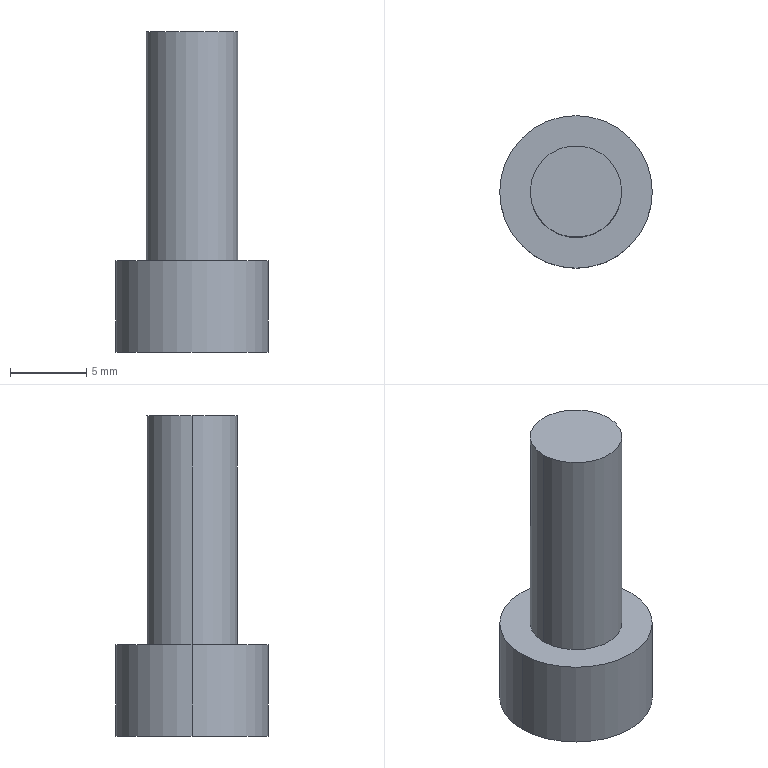Part | STEP file | LG M6_1.5F | 1 solid | 14 faces | box 10 x 10 x 21 mm | volume 829.881 mm3 | plane 10 | cylinder 4 | commonest cylinder face diameters 6 x2 10 x2
STEP:
#1=CARTESIAN_POINT('',(0.,0.,0.));
#2=DIRECTION('',(0.,0.,1.));
#3=DIRECTION('',(1.,0.,0.));
#4=AXIS2_PLACEMENT_3D('',#1,#2,#3);
#5=CARTESIAN_POINT('',(3.,0.,15.));
#6=VERTEX_POINT('',#5);
#7=CARTESIAN_POINT('',(-3.,0.,15.));
#8=VERTEX_POINT('',#7);
#9=CARTESIAN_POINT('',(0.,0.,15.));
#10=DIRECTION('',(0.,0.,1.));
#11=DIRECTION('',(1.,0.,0.));
#12=AXIS2_PLACEMENT_3D('',#9,#10,#11);
#13=CIRCLE('',#12,3.);
#14=CARTESIAN_POINT('',(0.,0.,15.));
#15=DIRECTION('',(0.,0.,-1.));
#16=DIRECTION('',(-1.,0.,0.));
#17=AXIS2_PLACEMENT_3D('',#14,#15,#16);
#18=CYLINDRICAL_SURFACE('',#17,3.);
#19=CARTESIAN_POINT('',(3.142,0.));
#20=DIRECTION('',(-1.,0.));
#21=VECTOR('',#20,1.);
#22=LINE('',#19,#21);
#23=(GEOMETRIC_REPRESENTATION_CONTEXT(2)PARAMETRIC_REPRESENTATION_CONTEXT()REPRESENTATION_CONTEXT('',''));
#24=DEFINITIONAL_REPRESENTATION('',(#22),#23);
#25=PCURVE('',#18,#24);
#26=CARTESIAN_POINT('',(0.,0.,15.));
#27=DIRECTION('',(0.,0.,1.));
#28=DIRECTION('',(1.,0.,0.));
#29=AXIS2_PLACEMENT_3D('',#26,#27,#28);
#30=PLANE('',#29);
#31=CARTESIAN_POINT('',(0.,0.));
#32=DIRECTION('',(1.,0.));
#33=AXIS2_PLACEMENT_2D('',#31,#32);
#34=CIRCLE('',#33,3.);
#35=(GEOMETRIC_REPRESENTATION_CONTEXT(2)PARAMETRIC_REPRESENTATION_CONTEXT()REPRESENTATION_CONTEXT('',''));
#36=DEFINITIONAL_REPRESENTATION('',(#34),#35);
#37=PCURVE('',#30,#36);
#38=SURFACE_CURVE('',#13,(#25,#37),.PCURVE_S1.);
#39=EDGE_CURVE('',#6,#8,#38,.T.);
#40=ORIENTED_EDGE('',*,*,#39,.F.);
#41=CARTESIAN_POINT('',(3.,0.,0.));
#42=VERTEX_POINT('',#41);
#43=CARTESIAN_POINT('',(3.,0.,15.));
#44=DIRECTION('',(0.,0.,-1.));
#45=VECTOR('',#44,1.);
#46=LINE('',#43,#45);
#47=CARTESIAN_POINT('',(3.142,0.));
#48=DIRECTION('',(0.,1.));
#49=VECTOR('',#48,1.);
#50=LINE('',#47,#49);
#51=(GEOMETRIC_REPRESENTATION_CONTEXT(2)PARAMETRIC_REPRESENTATION_CONTEXT()REPRESENTATION_CONTEXT('',''));
#52=DEFINITIONAL_REPRESENTATION('',(#50),#51);
#53=PCURVE('',#18,#52);
#54=CARTESIAN_POINT('',(0.,0.,15.));
#55=DIRECTION('',(0.,0.,-1.));
#56=DIRECTION('',(-1.,0.,0.));
#57=AXIS2_PLACEMENT_3D('',#54,#55,#56);
#58=CYLINDRICAL_SURFACE('',#57,3.);
#59=CARTESIAN_POINT('',(3.142,0.));
#60=DIRECTION('',(0.,1.));
#61=VECTOR('',#60,1.);
#62=LINE('',#59,#61);
#63=(GEOMETRIC_REPRESENTATION_CONTEXT(2)PARAMETRIC_REPRESENTATION_CONTEXT()REPRESENTATION_CONTEXT('',''));
#64=DEFINITIONAL_REPRESENTATION('',(#62),#63);
#65=PCURVE('',#58,#64);
#66=SURFACE_CURVE('',#46,(#53,#65),.PCURVE_S1.);
#67=EDGE_CURVE('',#6,#42,#66,.T.);
#68=ORIENTED_EDGE('',*,*,#67,.T.);
#69=CARTESIAN_POINT('',(-3.,0.,0.));
#70=VERTEX_POINT('',#69);
#71=CARTESIAN_POINT('',(0.,0.,0.));
#72=DIRECTION('',(0.,0.,1.));
#73=DIRECTION('',(1.,0.,0.));
#74=AXIS2_PLACEMENT_3D('',#71,#72,#73);
#75=CIRCLE('',#74,3.);
#76=CARTESIAN_POINT('',(3.142,15.));
#77=DIRECTION('',(-1.,0.));
#78=VECTOR('',#77,1.);
#79=LINE('',#76,#78);
#80=(GEOMETRIC_REPRESENTATION_CONTEXT(2)PARAMETRIC_REPRESENTATION_CONTEXT()REPRESENTATION_CONTEXT('',''));
#81=DEFINITIONAL_REPRESENTATION('',(#79),#80);
#82=PCURVE('',#18,#81);
#83=CARTESIAN_POINT('',(0.,0.,0.));
#84=DIRECTION('',(0.,0.,1.));
#85=DIRECTION('',(1.,0.,0.));
#86=AXIS2_PLACEMENT_3D('',#83,#84,#85);
#87=PLANE('',#86);
#88=CARTESIAN_POINT('',(0.,0.));
#89=DIRECTION('',(1.,0.));
#90=AXIS2_PLACEMENT_2D('',#88,#89);
#91=CIRCLE('',#90,3.);
#92=(GEOMETRIC_REPRESENTATION_CONTEXT(2)PARAMETRIC_REPRESENTATION_CONTEXT()REPRESENTATION_CONTEXT('',''));
#93=DEFINITIONAL_REPRESENTATION('',(#91),#92);
#94=PCURVE('',#87,#93);
#95=SURFACE_CURVE('',#75,(#82,#94),.PCURVE_S1.);
#96=EDGE_CURVE('',#42,#70,#95,.T.);
#97=ORIENTED_EDGE('',*,*,#96,.T.);
#98=CARTESIAN_POINT('',(-3.,0.,15.));
#99=DIRECTION('',(0.,0.,-1.));
#100=VECTOR('',#99,1.);
#101=LINE('',#98,#100);
#102=CARTESIAN_POINT('',(0.,0.));
#103=DIRECTION('',(0.,1.));
#104=VECTOR('',#103,1.);
#105=LINE('',#102,#104);
#106=(GEOMETRIC_REPRESENTATION_CONTEXT(2)PARAMETRIC_REPRESENTATION_CONTEXT()REPRESENTATION_CONTEXT('',''));
#107=DEFINITIONAL_REPRESENTATION('',(#105),#106);
#108=PCURVE('',#18,#107);
#109=CARTESIAN_POINT('',(6.283,0.));
#110=DIRECTION('',(0.,1.));
#111=VECTOR('',#110,1.);
#112=LINE('',#109,#111);
#113=(GEOMETRIC_REPRESENTATION_CONTEXT(2)PARAMETRIC_REPRESENTATION_CONTEXT()REPRESENTATION_CONTEXT('',''));
#114=DEFINITIONAL_REPRESENTATION('',(#112),#113);
#115=PCURVE('',#58,#114);
#116=SURFACE_CURVE('',#101,(#108,#115),.PCURVE_S1.);
#117=EDGE_CURVE('',#8,#70,#116,.T.);
#118=ORIENTED_EDGE('',*,*,#117,.F.);
#119=EDGE_LOOP('',(#40,#68,#97,#118));
#120=FACE_BOUND('',#119,.T.);
#121=ADVANCED_FACE('',(#120),#18,.T.);
#122=CARTESIAN_POINT('',(5.,0.,-6.));
#123=VERTEX_POINT('',#122);
#124=CARTESIAN_POINT('',(-5.,0.,-6.));
#125=VERTEX_POINT('',#124);
#126=CARTESIAN_POINT('',(0.,0.,-6.));
#127=DIRECTION('',(0.,0.,1.));
#128=DIRECTION('',(1.,0.,0.));
#129=AXIS2_PLACEMENT_3D('',#126,#127,#128);
#130=CIRCLE('',#129,5.);
#131=CARTESIAN_POINT('',(0.,0.,-6.));
#132=DIRECTION('',(0.,0.,1.));
#133=DIRECTION('',(1.,0.,0.));
#134=AXIS2_PLACEMENT_3D('',#131,#132,#133);
#135=CYLINDRICAL_SURFACE('',#134,5.);
#136=CARTESIAN_POINT('',(0.,0.));
#137=DIRECTION('',(1.,0.));
#138=VECTOR('',#137,1.);
#139=LINE('',#136,#138);
#140=(GEOMETRIC_REPRESENTATION_CONTEXT(2)PARAMETRIC_REPRESENTATION_CONTEXT()REPRESENTATION_CONTEXT('',''));
#141=DEFINITIONAL_REPRESENTATION('',(#139),#140);
#142=PCURVE('',#135,#141);
#143=CARTESIAN_POINT('',(0.,0.,-6.));
#144=DIRECTION('',(0.,0.,1.));
#145=DIRECTION('',(1.,0.,0.));
#146=AXIS2_PLACEMENT_3D('',#143,#144,#145);
#147=PLANE('',#146);
#148=CARTESIAN_POINT('',(0.,0.));
#149=DIRECTION('',(1.,0.));
#150=AXIS2_PLACEMENT_2D('',#148,#149);
#151=CIRCLE('',#150,5.);
#152=(GEOMETRIC_REPRESENTATION_CONTEXT(2)PARAMETRIC_REPRESENTATION_CONTEXT()REPRESENTATION_CONTEXT('',''));
#153=DEFINITIONAL_REPRESENTATION('',(#151),#152);
#154=PCURVE('',#147,#153);
#155=SURFACE_CURVE('',#130,(#142,#154),.PCURVE_S1.);
#156=EDGE_CURVE('',#123,#125,#155,.T.);
#157=ORIENTED_EDGE('',*,*,#156,.T.);
#158=CARTESIAN_POINT('',(-5.,0.,0.));
#159=VERTEX_POINT('',#158);
#160=CARTESIAN_POINT('',(-5.,0.,-6.));
#161=DIRECTION('',(0.,0.,1.));
#162=VECTOR('',#161,1.);
#163=LINE('',#160,#162);
#164=CARTESIAN_POINT('',(3.142,0.));
#165=DIRECTION('',(0.,1.));
#166=VECTOR('',#165,1.);
#167=LINE('',#164,#166);
#168=(GEOMETRIC_REPRESENTATION_CONTEXT(2)PARAMETRIC_REPRESENTATION_CONTEXT()REPRESENTATION_CONTEXT('',''));
#169=DEFINITIONAL_REPRESENTATION('',(#167),#168);
#170=PCURVE('',#135,#169);
#171=CARTESIAN_POINT('',(0.,0.,-6.));
#172=DIRECTION('',(0.,0.,1.));
#173=DIRECTION('',(1.,0.,0.));
#174=AXIS2_PLACEMENT_3D('',#171,#172,#173);
#175=CYLINDRICAL_SURFACE('',#174,5.);
#176=CARTESIAN_POINT('',(3.142,0.));
#177=DIRECTION('',(0.,1.));
#178=VECTOR('',#177,1.);
#179=LINE('',#176,#178);
#180=(GEOMETRIC_REPRESENTATION_CONTEXT(2)PARAMETRIC_REPRESENTATION_CONTEXT()REPRESENTATION_CONTEXT('',''));
#181=DEFINITIONAL_REPRESENTATION('',(#179),#180);
#182=PCURVE('',#175,#181);
#183=SURFACE_CURVE('',#163,(#170,#182),.PCURVE_S1.);
#184=EDGE_CURVE('',#125,#159,#183,.T.);
#185=ORIENTED_EDGE('',*,*,#184,.T.);
#186=CARTESIAN_POINT('',(5.,0.,0.));
#187=VERTEX_POINT('',#186);
#188=CARTESIAN_POINT('',(0.,0.,0.));
#189=DIRECTION('',(0.,0.,1.));
#190=DIRECTION('',(1.,0.,0.));
#191=AXIS2_PLACEMENT_3D('',#188,#189,#190);
#192=CIRCLE('',#191,5.);
#193=CARTESIAN_POINT('',(0.,6.));
#194=DIRECTION('',(1.,0.));
#195=VECTOR('',#194,1.);
#196=LINE('',#193,#195);
#197=(GEOMETRIC_REPRESENTATION_CONTEXT(2)PARAMETRIC_REPRESENTATION_CONTEXT()REPRESENTATION_CONTEXT('',''));
#198=DEFINITIONAL_REPRESENTATION('',(#196),#197);
#199=PCURVE('',#135,#198);
#200=CARTESIAN_POINT('',(0.,0.));
#201=DIRECTION('',(1.,0.));
#202=AXIS2_PLACEMENT_2D('',#200,#201);
#203=CIRCLE('',#202,5.);
#204=(GEOMETRIC_REPRESENTATION_CONTEXT(2)PARAMETRIC_REPRESENTATION_CONTEXT()REPRESENTATION_CONTEXT('',''));
#205=DEFINITIONAL_REPRESENTATION('',(#203),#204);
#206=PCURVE('',#87,#205);
#207=SURFACE_CURVE('',#192,(#199,#206),.PCURVE_S1.);
#208=EDGE_CURVE('',#187,#159,#207,.T.);
#209=ORIENTED_EDGE('',*,*,#208,.F.);
#210=CARTESIAN_POINT('',(5.,0.,-6.));
#211=DIRECTION('',(0.,0.,1.));
#212=VECTOR('',#211,1.);
#213=LINE('',#210,#212);
#214=CARTESIAN_POINT('',(0.,0.));
#215=DIRECTION('',(0.,1.));
#216=VECTOR('',#215,1.);
#217=LINE('',#214,#216);
#218=(GEOMETRIC_REPRESENTATION_CONTEXT(2)PARAMETRIC_REPRESENTATION_CONTEXT()REPRESENTATION_CONTEXT('',''));
#219=DEFINITIONAL_REPRESENTATION('',(#217),#218);
#220=PCURVE('',#135,#219);
#221=CARTESIAN_POINT('',(6.283,0.));
#222=DIRECTION('',(0.,1.));
#223=VECTOR('',#222,1.);
#224=LINE('',#221,#223);
#225=(GEOMETRIC_REPRESENTATION_CONTEXT(2)PARAMETRIC_REPRESENTATION_CONTEXT()REPRESENTATION_CONTEXT('',''));
#226=DEFINITIONAL_REPRESENTATION('',(#224),#225);
#227=PCURVE('',#175,#226);
#228=SURFACE_CURVE('',#213,(#220,#227),.PCURVE_S1.);
#229=EDGE_CURVE('',#123,#187,#228,.T.);
#230=ORIENTED_EDGE('',*,*,#229,.F.);
#231=EDGE_LOOP('',(#157,#185,#209,#230));
#232=FACE_BOUND('',#231,.T.);
#233=ADVANCED_FACE('',(#232),#135,.T.);
#234=ORIENTED_EDGE('',*,*,#208,.T.);
#235=CARTESIAN_POINT('',(0.,0.,0.));
#236=DIRECTION('',(0.,0.,1.));
#237=DIRECTION('',(1.,0.,0.));
#238=AXIS2_PLACEMENT_3D('',#235,#236,#237);
#239=CIRCLE('',#238,5.);
#240=CARTESIAN_POINT('',(0.,0.));
#241=DIRECTION('',(1.,0.));
#242=AXIS2_PLACEMENT_2D('',#240,#241);
#243=CIRCLE('',#242,5.);
#244=(GEOMETRIC_REPRESENTATION_CONTEXT(2)PARAMETRIC_REPRESENTATION_CONTEXT()REPRESENTATION_CONTEXT('',''));
#245=DEFINITIONAL_REPRESENTATION('',(#243),#244);
#246=PCURVE('',#87,#245);
#247=CARTESIAN_POINT('',(0.,6.));
#248=DIRECTION('',(1.,0.));
#249=VECTOR('',#248,1.);
#250=LINE('',#247,#249);
#251=(GEOMETRIC_REPRESENTATION_CONTEXT(2)PARAMETRIC_REPRESENTATION_CONTEXT()REPRESENTATION_CONTEXT('',''));
#252=DEFINITIONAL_REPRESENTATION('',(#250),#251);
#253=PCURVE('',#175,#252);
#254=SURFACE_CURVE('',#239,(#246,#253),.PCURVE_S1.);
#255=EDGE_CURVE('',#159,#187,#254,.T.);
#256=ORIENTED_EDGE('',*,*,#255,.T.);
#257=EDGE_LOOP('',(#234,#256));
#258=FACE_BOUND('',#257,.T.);
#259=CARTESIAN_POINT('',(0.,0.,0.));
#260=DIRECTION('',(0.,0.,1.));
#261=DIRECTION('',(1.,0.,0.));
#262=AXIS2_PLACEMENT_3D('',#259,#260,#261);
#263=CIRCLE('',#262,3.);
#264=CARTESIAN_POINT('',(0.,0.));
#265=DIRECTION('',(1.,0.));
#266=AXIS2_PLACEMENT_2D('',#264,#265);
#267=CIRCLE('',#266,3.);
#268=(GEOMETRIC_REPRESENTATION_CONTEXT(2)PARAMETRIC_REPRESENTATION_CONTEXT()REPRESENTATION_CONTEXT('',''));
#269=DEFINITIONAL_REPRESENTATION('',(#267),#268);
#270=PCURVE('',#87,#269);
#271=CARTESIAN_POINT('',(9.425,15.));
#272=DIRECTION('',(-1.,0.));
#273=VECTOR('',#272,1.);
#274=LINE('',#271,#273);
#275=(GEOMETRIC_REPRESENTATION_CONTEXT(2)PARAMETRIC_REPRESENTATION_CONTEXT()REPRESENTATION_CONTEXT('',''));
#276=DEFINITIONAL_REPRESENTATION('',(#274),#275);
#277=PCURVE('',#58,#276);
#278=SURFACE_CURVE('',#263,(#270,#277),.PCURVE_S1.);
#279=EDGE_CURVE('',#70,#42,#278,.T.);
#280=ORIENTED_EDGE('',*,*,#279,.F.);
#281=ORIENTED_EDGE('',*,*,#96,.F.);
#282=EDGE_LOOP('',(#280,#281));
#283=FACE_BOUND('',#282,.T.);
#284=ADVANCED_FACE('',(#258,#283),#87,.T.);
#285=ORIENTED_EDGE('',*,*,#184,.F.);
#286=CARTESIAN_POINT('',(0.,0.,-6.));
#287=DIRECTION('',(0.,0.,1.));
#288=DIRECTION('',(1.,0.,0.));
#289=AXIS2_PLACEMENT_3D('',#286,#287,#288);
#290=CIRCLE('',#289,5.);
#291=CARTESIAN_POINT('',(0.,0.));
#292=DIRECTION('',(1.,0.));
#293=VECTOR('',#292,1.);
#294=LINE('',#291,#293);
#295=(GEOMETRIC_REPRESENTATION_CONTEXT(2)PARAMETRIC_REPRESENTATION_CONTEXT()REPRESENTATION_CONTEXT('',''));
#296=DEFINITIONAL_REPRESENTATION('',(#294),#295);
#297=PCURVE('',#175,#296);
#298=CARTESIAN_POINT('',(0.,0.));
#299=DIRECTION('',(1.,0.));
#300=AXIS2_PLACEMENT_2D('',#298,#299);
#301=CIRCLE('',#300,5.);
#302=(GEOMETRIC_REPRESENTATION_CONTEXT(2)PARAMETRIC_REPRESENTATION_CONTEXT()REPRESENTATION_CONTEXT('',''));
#303=DEFINITIONAL_REPRESENTATION('',(#301),#302);
#304=PCURVE('',#147,#303);
#305=SURFACE_CURVE('',#290,(#297,#304),.PCURVE_S1.);
#306=EDGE_CURVE('',#125,#123,#305,.T.);
#307=ORIENTED_EDGE('',*,*,#306,.T.);
#308=ORIENTED_EDGE('',*,*,#229,.T.);
#309=ORIENTED_EDGE('',*,*,#255,.F.);
#310=EDGE_LOOP('',(#285,#307,#308,#309));
#311=FACE_BOUND('',#310,.T.);
#312=ADVANCED_FACE('',(#311),#175,.T.);
#313=CARTESIAN_POINT('',(-2.898,0.,-6.));
#314=VERTEX_POINT('',#313);
#315=CARTESIAN_POINT('',(-1.449,2.51,-6.));
#316=VERTEX_POINT('',#315);
#317=CARTESIAN_POINT('',(-2.898,0.,-6.));
#318=DIRECTION('',(0.5,0.866,0.));
#319=VECTOR('',#318,1.);
#320=LINE('',#317,#319);
#321=CARTESIAN_POINT('',(-2.898,0.));
#322=DIRECTION('',(0.5,0.866));
#323=VECTOR('',#322,1.);
#324=LINE('',#321,#323);
#325=(GEOMETRIC_REPRESENTATION_CONTEXT(2)PARAMETRIC_REPRESENTATION_CONTEXT()REPRESENTATION_CONTEXT('',''));
#326=DEFINITIONAL_REPRESENTATION('',(#324),#325);
#327=PCURVE('',#147,#326);
#328=CARTESIAN_POINT('',(-2.898,0.,-3.));
#329=DIRECTION('',(-0.866,0.5,0.));
#330=DIRECTION('',(-0.5,-0.866,0.));
#331=AXIS2_PLACEMENT_3D('',#328,#329,#330);
#332=PLANE('',#331);
#333=CARTESIAN_POINT('',(0.,-3.));
#334=DIRECTION('',(-1.,0.));
#335=VECTOR('',#334,1.);
#336=LINE('',#333,#335);
#337=(GEOMETRIC_REPRESENTATION_CONTEXT(2)PARAMETRIC_REPRESENTATION_CONTEXT()REPRESENTATION_CONTEXT('',''));
#338=DEFINITIONAL_REPRESENTATION('',(#336),#337);
#339=PCURVE('',#332,#338);
#340=SURFACE_CURVE('',#320,(#327,#339),.PCURVE_S1.);
#341=EDGE_CURVE('',#314,#316,#340,.T.);
#342=ORIENTED_EDGE('',*,*,#341,.F.);
#343=CARTESIAN_POINT('',(-1.449,-2.51,-6.));
#344=VERTEX_POINT('',#343);
#345=CARTESIAN_POINT('',(-1.449,-2.51,-6.));
#346=DIRECTION('',(-0.5,0.866,0.));
#347=VECTOR('',#346,1.);
#348=LINE('',#345,#347);
#349=CARTESIAN_POINT('',(-1.449,-2.51));
#350=DIRECTION('',(-0.5,0.866));
#351=VECTOR('',#350,1.);
#352=LINE('',#349,#351);
#353=(GEOMETRIC_REPRESENTATION_CONTEXT(2)PARAMETRIC_REPRESENTATION_CONTEXT()REPRESENTATION_CONTEXT('',''));
#354=DEFINITIONAL_REPRESENTATION('',(#352),#353);
#355=PCURVE('',#147,#354);
#356=CARTESIAN_POINT('',(-1.449,-2.51,-3.));
#357=DIRECTION('',(-0.866,-0.5,0.));
#358=DIRECTION('',(0.5,-0.866,0.));
#359=AXIS2_PLACEMENT_3D('',#356,#357,#358);
#360=PLANE('',#359);
#361=CARTESIAN_POINT('',(0.,-3.));
#362=DIRECTION('',(-1.,0.));
#363=VECTOR('',#362,1.);
#364=LINE('',#361,#363);
#365=(GEOMETRIC_REPRESENTATION_CONTEXT(2)PARAMETRIC_REPRESENTATION_CONTEXT()REPRESENTATION_CONTEXT('',''));
#366=DEFINITIONAL_REPRESENTATION('',(#364),#365);
#367=PCURVE('',#360,#366);
#368=SURFACE_CURVE('',#348,(#355,#367),.PCURVE_S1.);
#369=EDGE_CURVE('',#344,#314,#368,.T.);
#370=ORIENTED_EDGE('',*,*,#369,.F.);
#371=CARTESIAN_POINT('',(1.449,-2.51,-6.));
#372=VERTEX_POINT('',#371);
#373=CARTESIAN_POINT('',(1.449,-2.51,-6.));
#374=DIRECTION('',(-1.,0.,0.));
#375=VECTOR('',#374,1.);
#376=LINE('',#373,#375);
#377=CARTESIAN_POINT('',(1.449,-2.51));
#378=DIRECTION('',(-1.,0.));
#379=VECTOR('',#378,1.);
#380=LINE('',#377,#379);
#381=(GEOMETRIC_REPRESENTATION_CONTEXT(2)PARAMETRIC_REPRESENTATION_CONTEXT()REPRESENTATION_CONTEXT('',''));
#382=DEFINITIONAL_REPRESENTATION('',(#380),#381);
#383=PCURVE('',#147,#382);
#384=CARTESIAN_POINT('',(1.449,-2.51,-3.));
#385=DIRECTION('',(0.,-1.,0.));
#386=DIRECTION('',(0.,0.,-1.));
#387=AXIS2_PLACEMENT_3D('',#384,#385,#386);
#388=PLANE('',#387);
#389=CARTESIAN_POINT('',(3.,0.));
#390=DIRECTION('',(0.,-1.));
#391=VECTOR('',#390,1.);
#392=LINE('',#389,#391);
#393=(GEOMETRIC_REPRESENTATION_CONTEXT(2)PARAMETRIC_REPRESENTATION_CONTEXT()REPRESENTATION_CONTEXT('',''));
#394=DEFINITIONAL_REPRESENTATION('',(#392),#393);
#395=PCURVE('',#388,#394);
#396=SURFACE_CURVE('',#376,(#383,#395),.PCURVE_S1.);
#397=EDGE_CURVE('',#372,#344,#396,.T.);
#398=ORIENTED_EDGE('',*,*,#397,.F.);
#399=CARTESIAN_POINT('',(2.898,0.,-6.));
#400=VERTEX_POINT('',#399);
#401=CARTESIAN_POINT('',(2.898,0.,-6.));
#402=DIRECTION('',(-0.5,-0.866,0.));
#403=VECTOR('',#402,1.);
#404=LINE('',#401,#403);
#405=CARTESIAN_POINT('',(2.898,0.));
#406=DIRECTION('',(-0.5,-0.866));
#407=VECTOR('',#406,1.);
#408=LINE('',#405,#407);
#409=(GEOMETRIC_REPRESENTATION_CONTEXT(2)PARAMETRIC_REPRESENTATION_CONTEXT()REPRESENTATION_CONTEXT('',''));
#410=DEFINITIONAL_REPRESENTATION('',(#408),#409);
#411=PCURVE('',#147,#410);
#412=CARTESIAN_POINT('',(2.898,0.,-3.));
#413=DIRECTION('',(0.866,-0.5,0.));
#414=DIRECTION('',(0.5,0.866,0.));
#415=AXIS2_PLACEMENT_3D('',#412,#413,#414);
#416=PLANE('',#415);
#417=CARTESIAN_POINT('',(0.,-3.));
#418=DIRECTION('',(-1.,0.));
#419=VECTOR('',#418,1.);
#420=LINE('',#417,#419);
#421=(GEOMETRIC_REPRESENTATION_CONTEXT(2)PARAMETRIC_REPRESENTATION_CONTEXT()REPRESENTATION_CONTEXT('',''));
#422=DEFINITIONAL_REPRESENTATION('',(#420),#421);
#423=PCURVE('',#416,#422);
#424=SURFACE_CURVE('',#404,(#411,#423),.PCURVE_S1.);
#425=EDGE_CURVE('',#400,#372,#424,.T.);
#426=ORIENTED_EDGE('',*,*,#425,.F.);
#427=CARTESIAN_POINT('',(1.449,2.51,-6.));
#428=VERTEX_POINT('',#427);
#429=CARTESIAN_POINT('',(1.449,2.51,-6.));
#430=DIRECTION('',(0.5,-0.866,0.));
#431=VECTOR('',#430,1.);
#432=LINE('',#429,#431);
#433=CARTESIAN_POINT('',(1.449,2.51));
#434=DIRECTION('',(0.5,-0.866));
#435=VECTOR('',#434,1.);
#436=LINE('',#433,#435);
#437=(GEOMETRIC_REPRESENTATION_CONTEXT(2)PARAMETRIC_REPRESENTATION_CONTEXT()REPRESENTATION_CONTEXT('',''));
#438=DEFINITIONAL_REPRESENTATION('',(#436),#437);
#439=PCURVE('',#147,#438);
#440=CARTESIAN_POINT('',(1.449,2.51,-3.));
#441=DIRECTION('',(0.866,0.5,0.));
#442=DIRECTION('',(-0.5,0.866,0.));
#443=AXIS2_PLACEMENT_3D('',#440,#441,#442);
#444=PLANE('',#443);
#445=CARTESIAN_POINT('',(0.,-3.));
#446=DIRECTION('',(-1.,0.));
#447=VECTOR('',#446,1.);
#448=LINE('',#445,#447);
#449=(GEOMETRIC_REPRESENTATION_CONTEXT(2)PARAMETRIC_REPRESENTATION_CONTEXT()REPRESENTATION_CONTEXT('',''));
#450=DEFINITIONAL_REPRESENTATION('',(#448),#449);
#451=PCURVE('',#444,#450);
#452=SURFACE_CURVE('',#432,(#439,#451),.PCURVE_S1.);
#453=EDGE_CURVE('',#428,#400,#452,.T.);
#454=ORIENTED_EDGE('',*,*,#453,.F.);
#455=CARTESIAN_POINT('',(-1.449,2.51,-6.));
#456=DIRECTION('',(1.,0.,0.));
#457=VECTOR('',#456,1.);
#458=LINE('',#455,#457);
#459=CARTESIAN_POINT('',(-1.449,2.51));
#460=DIRECTION('',(1.,0.));
#461=VECTOR('',#460,1.);
#462=LINE('',#459,#461);
#463=(GEOMETRIC_REPRESENTATION_CONTEXT(2)PARAMETRIC_REPRESENTATION_CONTEXT()REPRESENTATION_CONTEXT('',''));
#464=DEFINITIONAL_REPRESENTATION('',(#462),#463);
#465=PCURVE('',#147,#464);
#466=CARTESIAN_POINT('',(-1.449,2.51,-3.));
#467=DIRECTION('',(0.,1.,0.));
#468=DIRECTION('',(0.,0.,1.));
#469=AXIS2_PLACEMENT_3D('',#466,#467,#468);
#470=PLANE('',#469);
#471=CARTESIAN_POINT('',(-3.,0.));
#472=DIRECTION('',(0.,1.));
#473=VECTOR('',#472,1.);
#474=LINE('',#471,#473);
#475=(GEOMETRIC_REPRESENTATION_CONTEXT(2)PARAMETRIC_REPRESENTATION_CONTEXT()REPRESENTATION_CONTEXT('',''));
#476=DEFINITIONAL_REPRESENTATION('',(#474),#475);
#477=PCURVE('',#470,#476);
#478=SURFACE_CURVE('',#458,(#465,#477),.PCURVE_S1.);
#479=EDGE_CURVE('',#316,#428,#478,.T.);
#480=ORIENTED_EDGE('',*,*,#479,.F.);
#481=EDGE_LOOP('',(#342,#370,#398,#426,#454,#480));
#482=FACE_BOUND('',#481,.T.);
#483=ORIENTED_EDGE('',*,*,#156,.F.);
#484=ORIENTED_EDGE('',*,*,#306,.F.);
#485=EDGE_LOOP('',(#483,#484));
#486=FACE_BOUND('',#485,.T.);
#487=ADVANCED_FACE('',(#482,#486),#147,.F.);
#488=ORIENTED_EDGE('',*,*,#67,.F.);
#489=CARTESIAN_POINT('',(0.,0.,15.));
#490=DIRECTION('',(0.,0.,1.));
#491=DIRECTION('',(1.,0.,0.));
#492=AXIS2_PLACEMENT_3D('',#489,#490,#491);
#493=CIRCLE('',#492,3.);
#494=CARTESIAN_POINT('',(9.425,0.));
#495=DIRECTION('',(-1.,0.));
#496=VECTOR('',#495,1.);
#497=LINE('',#494,#496);
#498=(GEOMETRIC_REPRESENTATION_CONTEXT(2)PARAMETRIC_REPRESENTATION_CONTEXT()REPRESENTATION_CONTEXT('',''));
#499=DEFINITIONAL_REPRESENTATION('',(#497),#498);
#500=PCURVE('',#58,#499);
#501=CARTESIAN_POINT('',(0.,0.));
#502=DIRECTION('',(1.,0.));
#503=AXIS2_PLACEMENT_2D('',#501,#502);
#504=CIRCLE('',#503,3.);
#505=(GEOMETRIC_REPRESENTATION_CONTEXT(2)PARAMETRIC_REPRESENTATION_CONTEXT()REPRESENTATION_CONTEXT('',''));
#506=DEFINITIONAL_REPRESENTATION('',(#504),#505);
#507=PCURVE('',#30,#506);
#508=SURFACE_CURVE('',#493,(#500,#507),.PCURVE_S1.);
#509=EDGE_CURVE('',#8,#6,#508,.T.);
#510=ORIENTED_EDGE('',*,*,#509,.F.);
#511=ORIENTED_EDGE('',*,*,#117,.T.);
#512=ORIENTED_EDGE('',*,*,#279,.T.);
#513=EDGE_LOOP('',(#488,#510,#511,#512));
#514=FACE_BOUND('',#513,.T.);
#515=ADVANCED_FACE('',(#514),#58,.T.);
#516=ORIENTED_EDGE('',*,*,#509,.T.);
#517=ORIENTED_EDGE('',*,*,#39,.T.);
#518=EDGE_LOOP('',(#516,#517));
#519=FACE_BOUND('',#518,.T.);
#520=ADVANCED_FACE('',(#519),#30,.T.);
#521=ORIENTED_EDGE('',*,*,#369,.T.);
#522=CARTESIAN_POINT('',(-2.898,0.,-3.));
#523=VERTEX_POINT('',#522);
#524=CARTESIAN_POINT('',(-2.898,0.,-3.));
#525=DIRECTION('',(0.,0.,-1.));
#526=VECTOR('',#525,1.);
#527=LINE('',#524,#526);
#528=CARTESIAN_POINT('',(-2.898,0.));
#529=DIRECTION('',(0.,-1.));
#530=VECTOR('',#529,1.);
#531=LINE('',#528,#530);
#532=(GEOMETRIC_REPRESENTATION_CONTEXT(2)PARAMETRIC_REPRESENTATION_CONTEXT()REPRESENTATION_CONTEXT('',''));
#533=DEFINITIONAL_REPRESENTATION('',(#531),#532);
#534=PCURVE('',#360,#533);
#535=CARTESIAN_POINT('',(0.,0.));
#536=DIRECTION('',(0.,-1.));
#537=VECTOR('',#536,1.);
#538=LINE('',#535,#537);
#539=(GEOMETRIC_REPRESENTATION_CONTEXT(2)PARAMETRIC_REPRESENTATION_CONTEXT()REPRESENTATION_CONTEXT('',''));
#540=DEFINITIONAL_REPRESENTATION('',(#538),#539);
#541=PCURVE('',#332,#540);
#542=SURFACE_CURVE('',#527,(#534,#541),.PCURVE_S1.);
#543=EDGE_CURVE('',#523,#314,#542,.T.);
#544=ORIENTED_EDGE('',*,*,#543,.F.);
#545=CARTESIAN_POINT('',(-1.449,-2.51,-3.));
#546=VERTEX_POINT('',#545);
#547=CARTESIAN_POINT('',(-1.449,-2.51,-3.));
#548=DIRECTION('',(-0.5,0.866,0.));
#549=VECTOR('',#548,1.);
#550=LINE('',#547,#549);
#551=CARTESIAN_POINT('',(0.,0.));
#552=DIRECTION('',(-1.,0.));
#553=VECTOR('',#552,1.);
#554=LINE('',#551,#553);
#555=(GEOMETRIC_REPRESENTATION_CONTEXT(2)PARAMETRIC_REPRESENTATION_CONTEXT()REPRESENTATION_CONTEXT('',''));
#556=DEFINITIONAL_REPRESENTATION('',(#554),#555);
#557=PCURVE('',#360,#556);
#558=CARTESIAN_POINT('',(0.,0.,-3.));
#559=DIRECTION('',(0.,0.,-1.));
#560=DIRECTION('',(-1.,0.,0.));
#561=AXIS2_PLACEMENT_3D('',#558,#559,#560);
#562=PLANE('',#561);
#563=CARTESIAN_POINT('',(1.449,-2.51));
#564=DIRECTION('',(0.5,0.866));
#565=VECTOR('',#564,1.);
#566=LINE('',#563,#565);
#567=(GEOMETRIC_REPRESENTATION_CONTEXT(2)PARAMETRIC_REPRESENTATION_CONTEXT()REPRESENTATION_CONTEXT('',''));
#568=DEFINITIONAL_REPRESENTATION('',(#566),#567);
#569=PCURVE('',#562,#568);
#570=SURFACE_CURVE('',#550,(#557,#569),.PCURVE_S1.);
#571=EDGE_CURVE('',#546,#523,#570,.T.);
#572=ORIENTED_EDGE('',*,*,#571,.F.);
#573=CARTESIAN_POINT('',(-1.449,-2.51,-3.));
#574=DIRECTION('',(0.,0.,-1.));
#575=VECTOR('',#574,1.);
#576=LINE('',#573,#575);
#577=CARTESIAN_POINT('',(0.,0.));
#578=DIRECTION('',(0.,-1.));
#579=VECTOR('',#578,1.);
#580=LINE('',#577,#579);
#581=(GEOMETRIC_REPRESENTATION_CONTEXT(2)PARAMETRIC_REPRESENTATION_CONTEXT()REPRESENTATION_CONTEXT('',''));
#582=DEFINITIONAL_REPRESENTATION('',(#580),#581);
#583=PCURVE('',#360,#582);
#584=CARTESIAN_POINT('',(0.,-2.898));
#585=DIRECTION('',(1.,0.));
#586=VECTOR('',#585,1.);
#587=LINE('',#584,#586);
#588=(GEOMETRIC_REPRESENTATION_CONTEXT(2)PARAMETRIC_REPRESENTATION_CONTEXT()REPRESENTATION_CONTEXT('',''));
#589=DEFINITIONAL_REPRESENTATION('',(#587),#588);
#590=PCURVE('',#388,#589);
#591=SURFACE_CURVE('',#576,(#583,#590),.PCURVE_S1.);
#592=EDGE_CURVE('',#546,#344,#591,.T.);
#593=ORIENTED_EDGE('',*,*,#592,.T.);
#594=EDGE_LOOP('',(#521,#544,#572,#593));
#595=FACE_BOUND('',#594,.T.);
#596=ADVANCED_FACE('',(#595),#360,.F.);
#597=ORIENTED_EDGE('',*,*,#397,.T.);
#598=ORIENTED_EDGE('',*,*,#592,.F.);
#599=CARTESIAN_POINT('',(1.449,-2.51,-3.));
#600=VERTEX_POINT('',#599);
#601=CARTESIAN_POINT('',(1.449,-2.51,-3.));
#602=DIRECTION('',(-1.,0.,0.));
#603=VECTOR('',#602,1.);
#604=LINE('',#601,#603);
#605=CARTESIAN_POINT('',(0.,0.));
#606=DIRECTION('',(0.,-1.));
#607=VECTOR('',#606,1.);
#608=LINE('',#605,#607);
#609=(GEOMETRIC_REPRESENTATION_CONTEXT(2)PARAMETRIC_REPRESENTATION_CONTEXT()REPRESENTATION_CONTEXT('',''));
#610=DEFINITIONAL_REPRESENTATION('',(#608),#609);
#611=PCURVE('',#388,#610);
#612=CARTESIAN_POINT('',(-1.449,-2.51));
#613=DIRECTION('',(1.,0.));
#614=VECTOR('',#613,1.);
#615=LINE('',#612,#614);
#616=(GEOMETRIC_REPRESENTATION_CONTEXT(2)PARAMETRIC_REPRESENTATION_CONTEXT()REPRESENTATION_CONTEXT('',''));
#617=DEFINITIONAL_REPRESENTATION('',(#615),#616);
#618=PCURVE('',#562,#617);
#619=SURFACE_CURVE('',#604,(#611,#618),.PCURVE_S1.);
#620=EDGE_CURVE('',#600,#546,#619,.T.);
#621=ORIENTED_EDGE('',*,*,#620,.F.);
#622=CARTESIAN_POINT('',(1.449,-2.51,-3.));
#623=DIRECTION('',(0.,0.,-1.));
#624=VECTOR('',#623,1.);
#625=LINE('',#622,#624);
#626=CARTESIAN_POINT('',(0.,0.));
#627=DIRECTION('',(1.,0.));
#628=VECTOR('',#627,1.);
#629=LINE('',#626,#628);
#630=(GEOMETRIC_REPRESENTATION_CONTEXT(2)PARAMETRIC_REPRESENTATION_CONTEXT()REPRESENTATION_CONTEXT('',''));
#631=DEFINITIONAL_REPRESENTATION('',(#629),#630);
#632=PCURVE('',#388,#631);
#633=CARTESIAN_POINT('',(-2.898,0.));
#634=DIRECTION('',(0.,-1.));
#635=VECTOR('',#634,1.);
#636=LINE('',#633,#635);
#637=(GEOMETRIC_REPRESENTATION_CONTEXT(2)PARAMETRIC_REPRESENTATION_CONTEXT()REPRESENTATION_CONTEXT('',''));
#638=DEFINITIONAL_REPRESENTATION('',(#636),#637);
#639=PCURVE('',#416,#638);
#640=SURFACE_CURVE('',#625,(#632,#639),.PCURVE_S1.);
#641=EDGE_CURVE('',#600,#372,#640,.T.);
#642=ORIENTED_EDGE('',*,*,#641,.T.);
#643=EDGE_LOOP('',(#597,#598,#621,#642));
#644=FACE_BOUND('',#643,.T.);
#645=ADVANCED_FACE('',(#644),#388,.F.);
#646=ORIENTED_EDGE('',*,*,#425,.T.);
#647=ORIENTED_EDGE('',*,*,#641,.F.);
#648=CARTESIAN_POINT('',(2.898,0.,-3.));
#649=VERTEX_POINT('',#648);
#650=CARTESIAN_POINT('',(2.898,0.,-3.));
#651=DIRECTION('',(-0.5,-0.866,0.));
#652=VECTOR('',#651,1.);
#653=LINE('',#650,#652);
#654=CARTESIAN_POINT('',(0.,0.));
#655=DIRECTION('',(-1.,0.));
#656=VECTOR('',#655,1.);
#657=LINE('',#654,#656);
#658=(GEOMETRIC_REPRESENTATION_CONTEXT(2)PARAMETRIC_REPRESENTATION_CONTEXT()REPRESENTATION_CONTEXT('',''));
#659=DEFINITIONAL_REPRESENTATION('',(#657),#658);
#660=PCURVE('',#416,#659);
#661=CARTESIAN_POINT('',(-2.898,0.));
#662=DIRECTION('',(0.5,-0.866));
#663=VECTOR('',#662,1.);
#664=LINE('',#661,#663);
#665=(GEOMETRIC_REPRESENTATION_CONTEXT(2)PARAMETRIC_REPRESENTATION_CONTEXT()REPRESENTATION_CONTEXT('',''));
#666=DEFINITIONAL_REPRESENTATION('',(#664),#665);
#667=PCURVE('',#562,#666);
#668=SURFACE_CURVE('',#653,(#660,#667),.PCURVE_S1.);
#669=EDGE_CURVE('',#649,#600,#668,.T.);
#670=ORIENTED_EDGE('',*,*,#669,.F.);
#671=CARTESIAN_POINT('',(2.898,0.,-3.));
#672=DIRECTION('',(0.,0.,-1.));
#673=VECTOR('',#672,1.);
#674=LINE('',#671,#673);
#675=CARTESIAN_POINT('',(0.,0.));
#676=DIRECTION('',(0.,-1.));
#677=VECTOR('',#676,1.);
#678=LINE('',#675,#677);
#679=(GEOMETRIC_REPRESENTATION_CONTEXT(2)PARAMETRIC_REPRESENTATION_CONTEXT()REPRESENTATION_CONTEXT('',''));
#680=DEFINITIONAL_REPRESENTATION('',(#678),#679);
#681=PCURVE('',#416,#680);
#682=CARTESIAN_POINT('',(-2.898,0.));
#683=DIRECTION('',(0.,-1.));
#684=VECTOR('',#683,1.);
#685=LINE('',#682,#684);
#686=(GEOMETRIC_REPRESENTATION_CONTEXT(2)PARAMETRIC_REPRESENTATION_CONTEXT()REPRESENTATION_CONTEXT('',''));
#687=DEFINITIONAL_REPRESENTATION('',(#685),#686);
#688=PCURVE('',#444,#687);
#689=SURFACE_CURVE('',#674,(#681,#688),.PCURVE_S1.);
#690=EDGE_CURVE('',#649,#400,#689,.T.);
#691=ORIENTED_EDGE('',*,*,#690,.T.);
#692=EDGE_LOOP('',(#646,#647,#670,#691));
#693=FACE_BOUND('',#692,.T.);
#694=ADVANCED_FACE('',(#693),#416,.F.);
#695=ORIENTED_EDGE('',*,*,#453,.T.);
#696=ORIENTED_EDGE('',*,*,#690,.F.);
#697=CARTESIAN_POINT('',(1.449,2.51,-3.));
#698=VERTEX_POINT('',#697);
#699=CARTESIAN_POINT('',(1.449,2.51,-3.));
#700=DIRECTION('',(0.5,-0.866,0.));
#701=VECTOR('',#700,1.);
#702=LINE('',#699,#701);
#703=CARTESIAN_POINT('',(0.,0.));
#704=DIRECTION('',(-1.,0.));
#705=VECTOR('',#704,1.);
#706=LINE('',#703,#705);
#707=(GEOMETRIC_REPRESENTATION_CONTEXT(2)PARAMETRIC_REPRESENTATION_CONTEXT()REPRESENTATION_CONTEXT('',''));
#708=DEFINITIONAL_REPRESENTATION('',(#706),#707);
#709=PCURVE('',#444,#708);
#710=CARTESIAN_POINT('',(-1.449,2.51));
#711=DIRECTION('',(-0.5,-0.866));
#712=VECTOR('',#711,1.);
#713=LINE('',#710,#712);
#714=(GEOMETRIC_REPRESENTATION_CONTEXT(2)PARAMETRIC_REPRESENTATION_CONTEXT()REPRESENTATION_CONTEXT('',''));
#715=DEFINITIONAL_REPRESENTATION('',(#713),#714);
#716=PCURVE('',#562,#715);
#717=SURFACE_CURVE('',#702,(#709,#716),.PCURVE_S1.);
#718=EDGE_CURVE('',#698,#649,#717,.T.);
#719=ORIENTED_EDGE('',*,*,#718,.F.);
#720=CARTESIAN_POINT('',(1.449,2.51,-3.));
#721=DIRECTION('',(0.,0.,-1.));
#722=VECTOR('',#721,1.);
#723=LINE('',#720,#722);
#724=CARTESIAN_POINT('',(0.,0.));
#725=DIRECTION('',(0.,-1.));
#726=VECTOR('',#725,1.);
#727=LINE('',#724,#726);
#728=(GEOMETRIC_REPRESENTATION_CONTEXT(2)PARAMETRIC_REPRESENTATION_CONTEXT()REPRESENTATION_CONTEXT('',''));
#729=DEFINITIONAL_REPRESENTATION('',(#727),#728);
#730=PCURVE('',#444,#729);
#731=CARTESIAN_POINT('',(0.,2.898));
#732=DIRECTION('',(-1.,0.));
#733=VECTOR('',#732,1.);
#734=LINE('',#731,#733);
#735=(GEOMETRIC_REPRESENTATION_CONTEXT(2)PARAMETRIC_REPRESENTATION_CONTEXT()REPRESENTATION_CONTEXT('',''));
#736=DEFINITIONAL_REPRESENTATION('',(#734),#735);
#737=PCURVE('',#470,#736);
#738=SURFACE_CURVE('',#723,(#730,#737),.PCURVE_S1.);
#739=EDGE_CURVE('',#698,#428,#738,.T.);
#740=ORIENTED_EDGE('',*,*,#739,.T.);
#741=EDGE_LOOP('',(#695,#696,#719,#740));
#742=FACE_BOUND('',#741,.T.);
#743=ADVANCED_FACE('',(#742),#444,.F.);
#744=ORIENTED_EDGE('',*,*,#479,.T.);
#745=ORIENTED_EDGE('',*,*,#739,.F.);
#746=CARTESIAN_POINT('',(-1.449,2.51,-3.));
#747=VERTEX_POINT('',#746);
#748=CARTESIAN_POINT('',(-1.449,2.51,-3.));
#749=DIRECTION('',(1.,0.,0.));
#750=VECTOR('',#749,1.);
#751=LINE('',#748,#750);
#752=CARTESIAN_POINT('',(0.,0.));
#753=DIRECTION('',(0.,1.));
#754=VECTOR('',#753,1.);
#755=LINE('',#752,#754);
#756=(GEOMETRIC_REPRESENTATION_CONTEXT(2)PARAMETRIC_REPRESENTATION_CONTEXT()REPRESENTATION_CONTEXT('',''));
#757=DEFINITIONAL_REPRESENTATION('',(#755),#756);
#758=PCURVE('',#470,#757);
#759=CARTESIAN_POINT('',(1.449,2.51));
#760=DIRECTION('',(-1.,0.));
#761=VECTOR('',#760,1.);
#762=LINE('',#759,#761);
#763=(GEOMETRIC_REPRESENTATION_CONTEXT(2)PARAMETRIC_REPRESENTATION_CONTEXT()REPRESENTATION_CONTEXT('',''));
#764=DEFINITIONAL_REPRESENTATION('',(#762),#763);
#765=PCURVE('',#562,#764);
#766=SURFACE_CURVE('',#751,(#758,#765),.PCURVE_S1.);
#767=EDGE_CURVE('',#747,#698,#766,.T.);
#768=ORIENTED_EDGE('',*,*,#767,.F.);
#769=CARTESIAN_POINT('',(-1.449,2.51,-3.));
#770=DIRECTION('',(0.,0.,-1.));
#771=VECTOR('',#770,1.);
#772=LINE('',#769,#771);
#773=CARTESIAN_POINT('',(0.,0.));
#774=DIRECTION('',(-1.,0.));
#775=VECTOR('',#774,1.);
#776=LINE('',#773,#775);
#777=(GEOMETRIC_REPRESENTATION_CONTEXT(2)PARAMETRIC_REPRESENTATION_CONTEXT()REPRESENTATION_CONTEXT('',''));
#778=DEFINITIONAL_REPRESENTATION('',(#776),#777);
#779=PCURVE('',#470,#778);
#780=CARTESIAN_POINT('',(-2.898,0.));
#781=DIRECTION('',(0.,-1.));
#782=VECTOR('',#781,1.);
#783=LINE('',#780,#782);
#784=(GEOMETRIC_REPRESENTATION_CONTEXT(2)PARAMETRIC_REPRESENTATION_CONTEXT()REPRESENTATION_CONTEXT('',''));
#785=DEFINITIONAL_REPRESENTATION('',(#783),#784);
#786=PCURVE('',#332,#785);
#787=SURFACE_CURVE('',#772,(#779,#786),.PCURVE_S1.);
#788=EDGE_CURVE('',#747,#316,#787,.T.);
#789=ORIENTED_EDGE('',*,*,#788,.T.);
#790=EDGE_LOOP('',(#744,#745,#768,#789));
#791=FACE_BOUND('',#790,.T.);
#792=ADVANCED_FACE('',(#791),#470,.F.);
#793=ORIENTED_EDGE('',*,*,#341,.T.);
#794=ORIENTED_EDGE('',*,*,#788,.F.);
#795=CARTESIAN_POINT('',(-2.898,0.,-3.));
#796=DIRECTION('',(0.5,0.866,0.));
#797=VECTOR('',#796,1.);
#798=LINE('',#795,#797);
#799=CARTESIAN_POINT('',(0.,0.));
#800=DIRECTION('',(-1.,0.));
#801=VECTOR('',#800,1.);
#802=LINE('',#799,#801);
#803=(GEOMETRIC_REPRESENTATION_CONTEXT(2)PARAMETRIC_REPRESENTATION_CONTEXT()REPRESENTATION_CONTEXT('',''));
#804=DEFINITIONAL_REPRESENTATION('',(#802),#803);
#805=PCURVE('',#332,#804);
#806=CARTESIAN_POINT('',(2.898,0.));
#807=DIRECTION('',(-0.5,0.866));
#808=VECTOR('',#807,1.);
#809=LINE('',#806,#808);
#810=(GEOMETRIC_REPRESENTATION_CONTEXT(2)PARAMETRIC_REPRESENTATION_CONTEXT()REPRESENTATION_CONTEXT('',''));
#811=DEFINITIONAL_REPRESENTATION('',(#809),#810);
#812=PCURVE('',#562,#811);
#813=SURFACE_CURVE('',#798,(#805,#812),.PCURVE_S1.);
#814=EDGE_CURVE('',#523,#747,#813,.T.);
#815=ORIENTED_EDGE('',*,*,#814,.F.);
#816=ORIENTED_EDGE('',*,*,#543,.T.);
#817=EDGE_LOOP('',(#793,#794,#815,#816));
#818=FACE_BOUND('',#817,.T.);
#819=ADVANCED_FACE('',(#818),#332,.F.);
#820=ORIENTED_EDGE('',*,*,#571,.T.);
#821=ORIENTED_EDGE('',*,*,#814,.T.);
#822=ORIENTED_EDGE('',*,*,#767,.T.);
#823=ORIENTED_EDGE('',*,*,#718,.T.);
#824=ORIENTED_EDGE('',*,*,#669,.T.);
#825=ORIENTED_EDGE('',*,*,#620,.T.);
#826=EDGE_LOOP('',(#820,#821,#822,#823,#824,#825));
#827=FACE_BOUND('',#826,.T.);
#828=ADVANCED_FACE('',(#827),#562,.T.);
#829=CLOSED_SHELL('',(#121,#233,#284,#312,#487,#515,#520,#596,#645,#694,#743,#792,#819,#828));
#830=MANIFOLD_SOLID_BREP('',#829);
#831=(LENGTH_UNIT()NAMED_UNIT(*)SI_UNIT(.MILLI.,.METRE.));
#832=UNCERTAINTY_MEASURE_WITH_UNIT(LENGTH_MEASURE(0.0000001),#831,'','');
#833=(NAMED_UNIT(*)PLANE_ANGLE_UNIT()SI_UNIT($,.RADIAN.));
#834=(NAMED_UNIT(*)SI_UNIT($,.STERADIAN.)SOLID_ANGLE_UNIT());
#835=(GEOMETRIC_REPRESENTATION_CONTEXT(3)GLOBAL_UNCERTAINTY_ASSIGNED_CONTEXT((#832))GLOBAL_UNIT_ASSIGNED_CONTEXT((#831,#833,#834))REPRESENTATION_CONTEXT('',''));
#836=ADVANCED_BREP_SHAPE_REPRESENTATION('',(#4,#830),#835);